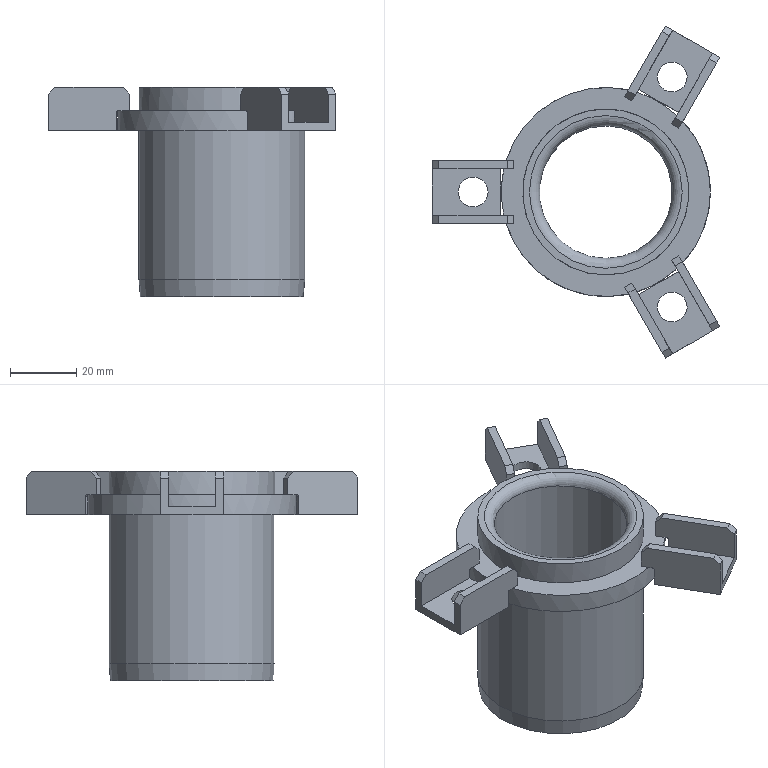Part | STEP file | gslz 2016.10.28-6_id838_x_t | 1 solid | 74 faces | box 86.634 x 100.036 x 63 mm | volume 56971 mm3 | plane 58 | cylinder 13 | torus 2 | cone 1 | commonest cylinder face diameters 1 x6 9 x3 50 x2 40 x1 63 x1